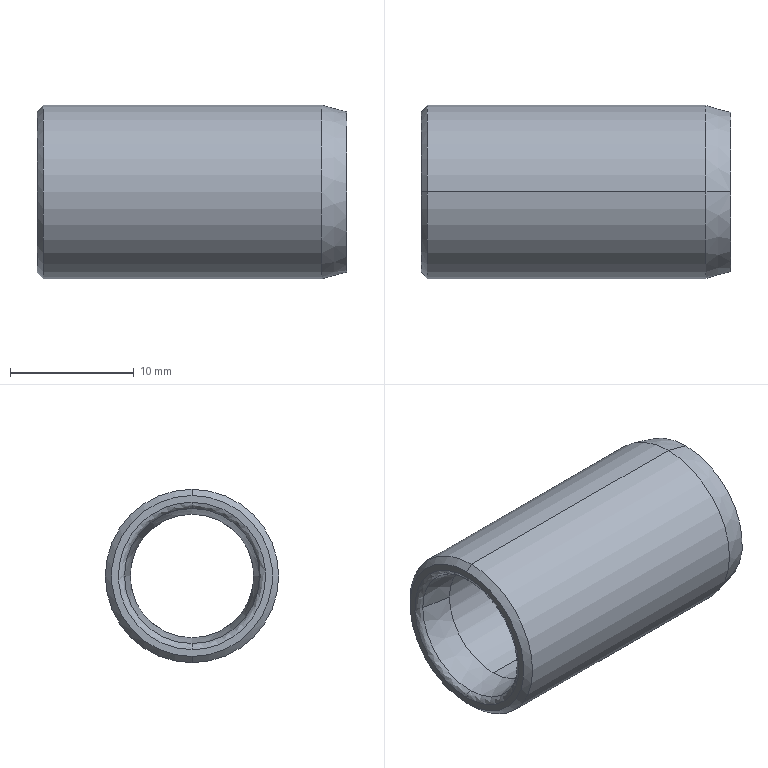Part | STEP file | OFK01-d10-L25 | 1 solid | 18 faces | box 25 x 14 x 14 mm | volume 1804 mm3 | cone 8 | spline 4 | cylinder 4 | plane 2 | commonest cylinder face diameters 10 x2 14 x2